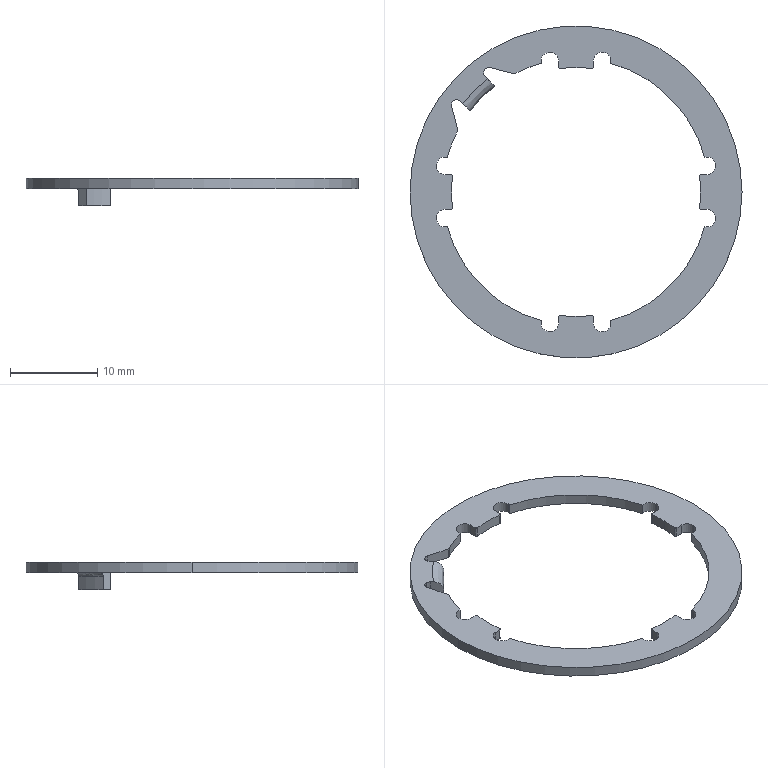Part | SolidWorks | features RefAxis 3, BaseBody 1 | 1 solid | 66 faces | box 38 x 38 x 3.2 mm | volume 486.379 mm3 | cylinder 48 | plane 15 | spline 3 | commonest cylinder face diameters 30.5 x14 0.4 x12 2 x12 28.5 x5 1.227 x2 38 x2